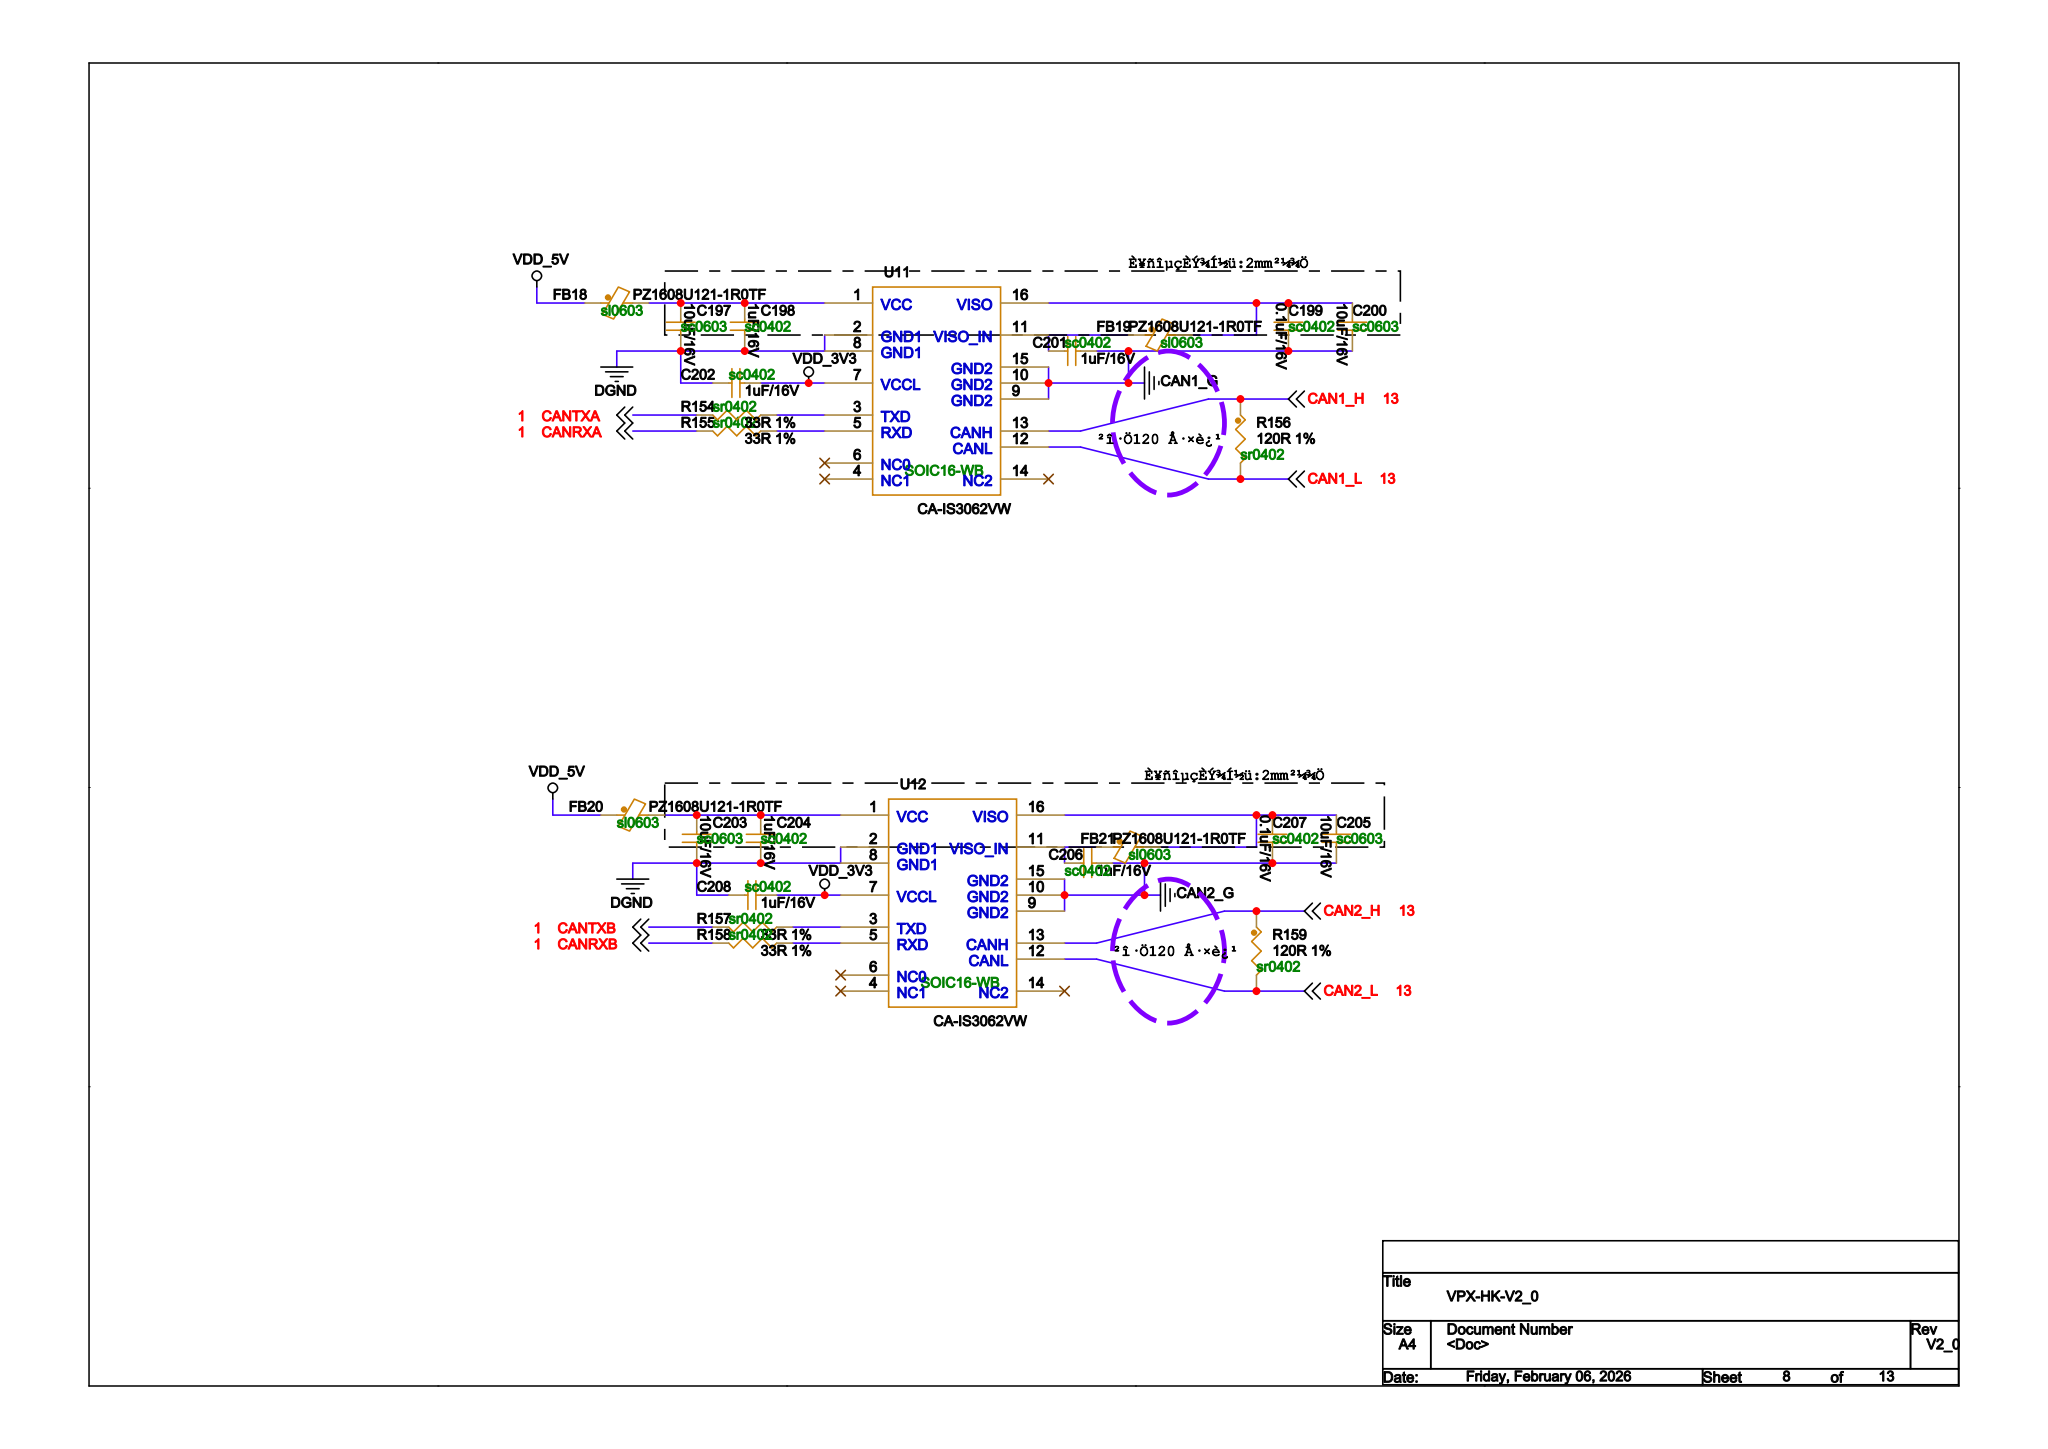Circuit board | Cadence Allegro | 598 parts | 541 nets | one sheet of the schematic
Parts on this sheet (reference | value | footprint):
C197 | 10uF/16V | SC0603
C198 | 1uF/16V | SC0402
C199 | 0.1uF/16V | SC0402
C200 | 10uF/16V | SC0603
C201 | 1uF/16V | SC0402
C202 | 1uF/16V | SC0402
C203 | 10uF/16V | SC0603
C204 | 1uF/16V | SC0402
C205 | 10uF/16V | SC0603
C206 | 1uF/16V | SC0402
C207 | 0.1uF/16V | SC0402
C208 | 1uF/16V | SC0402
FB18 | PZ1608U121-1R0TF | SL0603
FB20 | PZ1608U121-1R0TF | SL0603
R154 | 33R 1% | SR0402
R155 | 33R 1% | SR0402
R156 | 120R 1% | SR0402
R157 | 33R 1% | SR0402
R158 | 33R 1% | SR0402
R159 | 120R 1% | SR0402
U11 | CA-IS3062VW | SOIC16-WB
U12 | CA-IS3062VW | SOIC16-WB
Nets of these parts (net: part-pin ...):
DGND: C197-2 C198-2 C202-1 C203-2 C204-2 C208-1 U11-2 U11-8 U12-2 U12-8
VDD_5V: FB18-1 FB20-1
VDD_3V3: C202-2 C208-2 U11-7 U12-7
N33397823: C199-1 C200-1 U11-16
CAN1_G: C199-2 C200-2 C201-2 U11-9 U11-10 U11-15
N33395360: C205-1 C207-1 U12-16
CAN2_G: C205-2 C206-2 C207-2 U12-9 U12-10 U12-15
N33397665: C201-1 U11-11
N33395192: C206-1 U12-11
N33397709: C197-1 C198-1 FB18-2 U11-1
N33395246: C203-1 C204-1 FB20-2 U12-1
CAN1_H: R156-1 U11-13
CAN1_L: R156-2 U11-12
CAN2_H: R159-1 U12-13
CAN2_L: R159-2 U12-12
CANTXA: R154-1
N33397633: R154-2 U11-3
CANRXA: R155-1
N33397635: R155-2 U11-5
CANTXB: R157-1
N33396687: R157-2 U12-3
CANRXB: R158-1
N33396709: R158-2 U12-5